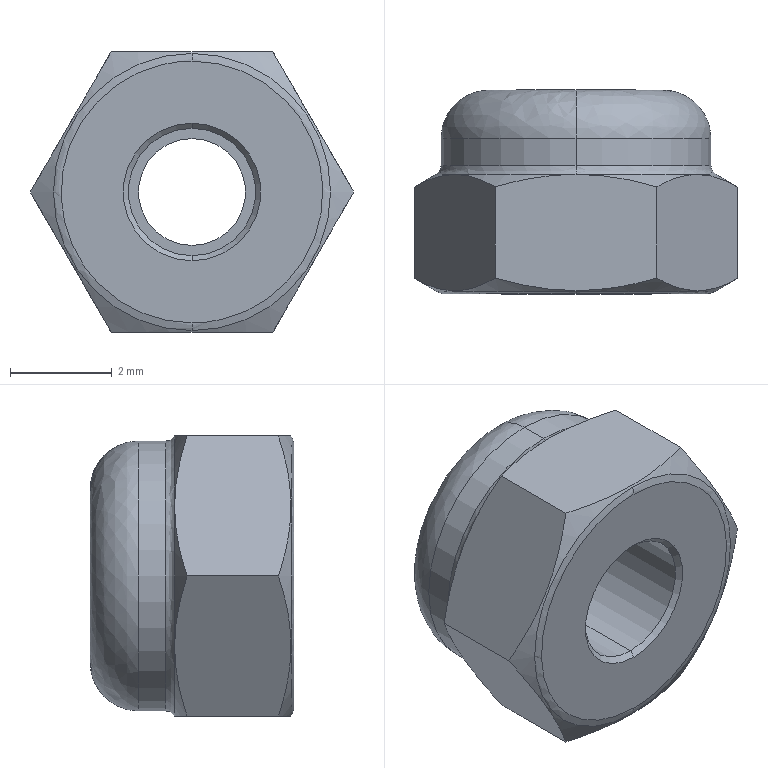Part | SolidWorks | features BaseBody 1 | 1 solid | 39 faces | box 6.351 x 4 x 5.5 mm | volume 76.032 mm3 | plane 11 | cone 10 | cylinder 10 | spline 8 | commonest cylinder face diameters 2.1 x2 2.5 x2 3 x2 4 x2 5.3 x2
STEP:
#1=CARTESIAN_POINT('',(0.,-1.16,2.72));
#2=VERTEX_POINT('',#1);
#3=CARTESIAN_POINT('',(0.,-1.16,-2.72));
#4=VERTEX_POINT('',#3);
#5=CARTESIAN_POINT('',(0.,-1.16,0.));
#6=DIRECTION('',(0.,-1.,0.));
#7=DIRECTION('',(0.,0.,1.));
#8=AXIS2_PLACEMENT_3D('',#5,#6,#7);
#9=CIRCLE('',#8,2.72);
#10=EDGE_CURVE('',#2,#4,#9,.T.);
#11=ORIENTED_EDGE('',*,*,#10,.T.);
#12=CARTESIAN_POINT('',(0.,-1.2,-2.57));
#13=VERTEX_POINT('',#12);
#14=CARTESIAN_POINT('',(0.,-0.9,-2.57));
#15=DIRECTION('',(-1.,0.,0.));
#16=DIRECTION('',(0.,0.,-1.));
#17=AXIS2_PLACEMENT_3D('',#14,#15,#16);
#18=CIRCLE('',#17,0.3);
#19=EDGE_CURVE('',#4,#13,#18,.T.);
#20=ORIENTED_EDGE('',*,*,#19,.T.);
#21=CARTESIAN_POINT('',(0.,-1.2,2.57));
#22=VERTEX_POINT('',#21);
#23=CARTESIAN_POINT('',(0.,-1.2,-2.57));
#24=CARTESIAN_POINT('',(-5.139,-1.2,-2.57));
#25=CARTESIAN_POINT('',(-5.139,-1.2,2.57));
#26=CARTESIAN_POINT('',(0.,-1.2,2.57));
#27=(BOUNDED_CURVE()B_SPLINE_CURVE(3,(#23,#24,#25,#26),.UNSPECIFIED.,.F.,.F.)B_SPLINE_CURVE_WITH_KNOTS((4,4),(0.,1.),.UNSPECIFIED.)CURVE()GEOMETRIC_REPRESENTATION_ITEM()RATIONAL_B_SPLINE_CURVE((1.,0.3333,0.3333,1.))REPRESENTATION_ITEM(''));
#28=EDGE_CURVE('',#13,#22,#27,.T.);
#29=ORIENTED_EDGE('',*,*,#28,.T.);
#30=CARTESIAN_POINT('',(0.,-0.9,2.57));
#31=DIRECTION('',(1.,0.,0.));
#32=DIRECTION('',(0.,0.,1.));
#33=AXIS2_PLACEMENT_3D('',#30,#31,#32);
#34=CIRCLE('',#33,0.3);
#35=EDGE_CURVE('',#2,#22,#34,.T.);
#36=ORIENTED_EDGE('',*,*,#35,.F.);
#37=EDGE_LOOP('',(#11,#20,#29,#36));
#38=FACE_OUTER_BOUND('',#37,.T.);
#39=CARTESIAN_POINT('',(0.,-1.16,-2.72));
#40=CARTESIAN_POINT('',(-5.439,-1.16,-2.72));
#41=CARTESIAN_POINT('',(-5.439,-1.16,2.72));
#42=CARTESIAN_POINT('',(0.,-1.16,2.72));
#43=CARTESIAN_POINT('',(0.,-1.186,-2.674));
#44=CARTESIAN_POINT('',(-5.347,-1.186,-2.674));
#45=CARTESIAN_POINT('',(-5.347,-1.186,2.674));
#46=CARTESIAN_POINT('',(0.,-1.186,2.674));
#47=CARTESIAN_POINT('',(0.,-1.2,-2.623));
#48=CARTESIAN_POINT('',(-5.245,-1.2,-2.623));
#49=CARTESIAN_POINT('',(-5.245,-1.2,2.623));
#50=CARTESIAN_POINT('',(0.,-1.2,2.623));
#51=CARTESIAN_POINT('',(0.,-1.2,-2.57));
#52=CARTESIAN_POINT('',(-5.139,-1.2,-2.57));
#53=CARTESIAN_POINT('',(-5.139,-1.2,2.57));
#54=CARTESIAN_POINT('',(0.,-1.2,2.57));
#55=(BOUNDED_SURFACE()B_SPLINE_SURFACE(3,3,((#39,#40,#41,#42),(#43,#44,#45,#46),(#47,#48,#49,#50),(#51,#52,#53,#54)),.UNSPECIFIED.,.F.,.F.,.F.)B_SPLINE_SURFACE_WITH_KNOTS((4,4),(4,4),(0.,1.),(0.,1.),.UNSPECIFIED.)GEOMETRIC_REPRESENTATION_ITEM()RATIONAL_B_SPLINE_SURFACE(((1.,0.3333,0.3333,1.),(0.9773,0.3258,0.3258,0.9773),(0.9773,0.3258,0.3258,0.9773),(1.,0.3333,0.3333,1.)))REPRESENTATION_ITEM('')SURFACE());
#56=ADVANCED_FACE('',(#38),#55,.T.);
#57=CARTESIAN_POINT('',(0.,1.142,-2.75));
#58=VERTEX_POINT('',#57);
#59=CARTESIAN_POINT('',(2.382,1.142,-1.375));
#60=VERTEX_POINT('',#59);
#61=CARTESIAN_POINT('',(0.,1.142,0.));
#62=DIRECTION('',(0.,-1.,0.));
#63=DIRECTION('',(0.,0.,-1.));
#64=AXIS2_PLACEMENT_3D('',#61,#62,#63);
#65=CIRCLE('',#64,2.75);
#66=EDGE_CURVE('',#58,#60,#65,.T.);
#67=ORIENTED_EDGE('',*,*,#66,.F.);
#68=CARTESIAN_POINT('',(0.,1.315,-2.65));
#69=VERTEX_POINT('',#68);
#70=CARTESIAN_POINT('',(0.,1.315,-2.85));
#71=DIRECTION('',(-1.,0.,0.));
#72=DIRECTION('',(0.,0.,-1.));
#73=AXIS2_PLACEMENT_3D('',#70,#71,#72);
#74=CIRCLE('',#73,0.2);
#75=EDGE_CURVE('',#58,#69,#74,.T.);
#76=ORIENTED_EDGE('',*,*,#75,.T.);
#77=CARTESIAN_POINT('',(0.,1.315,2.65));
#78=VERTEX_POINT('',#77);
#79=CARTESIAN_POINT('',(0.,1.315,0.));
#80=DIRECTION('',(0.,1.,0.));
#81=DIRECTION('',(0.,0.,1.));
#82=AXIS2_PLACEMENT_3D('',#79,#80,#81);
#83=CIRCLE('',#82,2.65);
#84=EDGE_CURVE('',#78,#69,#83,.T.);
#85=ORIENTED_EDGE('',*,*,#84,.F.);
#86=CARTESIAN_POINT('',(0.,1.142,2.75));
#87=VERTEX_POINT('',#86);
#88=CARTESIAN_POINT('',(0.,1.315,2.85));
#89=DIRECTION('',(1.,0.,0.));
#90=DIRECTION('',(0.,0.,1.));
#91=AXIS2_PLACEMENT_3D('',#88,#89,#90);
#92=CIRCLE('',#91,0.2);
#93=EDGE_CURVE('',#87,#78,#92,.T.);
#94=ORIENTED_EDGE('',*,*,#93,.F.);
#95=CARTESIAN_POINT('',(2.382,1.142,1.375));
#96=VERTEX_POINT('',#95);
#97=CARTESIAN_POINT('',(0.,1.142,0.));
#98=DIRECTION('',(0.,-1.,0.));
#99=DIRECTION('',(0.,0.,1.));
#100=AXIS2_PLACEMENT_3D('',#97,#98,#99);
#101=CIRCLE('',#100,2.75);
#102=EDGE_CURVE('',#96,#87,#101,.T.);
#103=ORIENTED_EDGE('',*,*,#102,.F.);
#104=CARTESIAN_POINT('',(0.,1.142,0.));
#105=DIRECTION('',(0.,-1.,0.));
#106=DIRECTION('',(0.,0.,1.));
#107=AXIS2_PLACEMENT_3D('',#104,#105,#106);
#108=CIRCLE('',#107,2.75);
#109=EDGE_CURVE('',#60,#96,#108,.T.);
#110=ORIENTED_EDGE('',*,*,#109,.F.);
#111=EDGE_LOOP('',(#67,#76,#85,#94,#103,#110));
#112=FACE_OUTER_BOUND('',#111,.T.);
#113=CARTESIAN_POINT('',(0.,1.142,2.75));
#114=CARTESIAN_POINT('',(5.5,1.142,2.75));
#115=CARTESIAN_POINT('',(5.5,1.142,-2.75));
#116=CARTESIAN_POINT('',(0.,1.142,-2.75));
#117=CARTESIAN_POINT('',(0.,1.179,2.687));
#118=CARTESIAN_POINT('',(5.373,1.179,2.687));
#119=CARTESIAN_POINT('',(5.373,1.179,-2.687));
#120=CARTESIAN_POINT('',(0.,1.179,-2.687));
#121=CARTESIAN_POINT('',(0.,1.242,2.65));
#122=CARTESIAN_POINT('',(5.3,1.242,2.65));
#123=CARTESIAN_POINT('',(5.3,1.242,-2.65));
#124=CARTESIAN_POINT('',(0.,1.242,-2.65));
#125=CARTESIAN_POINT('',(0.,1.315,2.65));
#126=CARTESIAN_POINT('',(5.3,1.315,2.65));
#127=CARTESIAN_POINT('',(5.3,1.315,-2.65));
#128=CARTESIAN_POINT('',(0.,1.315,-2.65));
#129=(BOUNDED_SURFACE()B_SPLINE_SURFACE(3,3,((#113,#114,#115,#116),(#117,#118,#119,#120),(#121,#122,#123,#124),(#125,#126,#127,#128)),.UNSPECIFIED.,.F.,.F.,.F.)B_SPLINE_SURFACE_WITH_KNOTS((4,4),(4,4),(0.,1.),(0.,1.),.UNSPECIFIED.)GEOMETRIC_REPRESENTATION_ITEM()RATIONAL_B_SPLINE_SURFACE(((1.,0.3333,0.3333,1.),(0.9107,0.3036,0.3036,0.9107),(0.9107,0.3036,0.3036,0.9107),(1.,0.3333,0.3333,1.)))REPRESENTATION_ITEM('')SURFACE());
#130=ADVANCED_FACE('',(#112),#129,.F.);
#131=CARTESIAN_POINT('',(0.,2.8,-1.7));
#132=VERTEX_POINT('',#131);
#133=CARTESIAN_POINT('',(0.,2.8,1.7));
#134=VERTEX_POINT('',#133);
#135=CARTESIAN_POINT('',(0.,2.8,-1.7));
#136=CARTESIAN_POINT('',(-0.108,2.8,-1.7));
#137=CARTESIAN_POINT('',(-0.2672,2.8,-1.685));
#138=CARTESIAN_POINT('',(-0.4481,2.8,-1.642));
#139=CARTESIAN_POINT('',(-0.5373,2.8,-1.613));
#140=CARTESIAN_POINT('',(-0.5753,2.8,-1.6));
#141=CARTESIAN_POINT('',(-0.6006,2.8,-1.59));
#142=CARTESIAN_POINT('',(-0.6121,2.8,-1.586));
#143=CARTESIAN_POINT('',(-0.8437,2.8,-1.494));
#144=CARTESIAN_POINT('',(-1.036,2.8,-1.368));
#145=CARTESIAN_POINT('',(-1.285,2.8,-1.119));
#146=CARTESIAN_POINT('',(-1.394,2.8,-0.9851));
#147=CARTESIAN_POINT('',(-1.496,2.8,-0.8112));
#148=CARTESIAN_POINT('',(-1.541,2.8,-0.7199));
#149=CARTESIAN_POINT('',(-1.558,2.8,-0.6799));
#150=CARTESIAN_POINT('',(-1.57,2.8,-0.653));
#151=CARTESIAN_POINT('',(-1.576,2.8,-0.6383));
#152=CARTESIAN_POINT('',(-1.66,2.8,-0.4251));
#153=CARTESIAN_POINT('',(-1.7,2.8,-0.2158));
#154=CARTESIAN_POINT('',(-1.7,2.8,0.1079));
#155=CARTESIAN_POINT('',(-1.685,2.8,0.2671));
#156=CARTESIAN_POINT('',(-1.642,2.8,0.448));
#157=CARTESIAN_POINT('',(-1.617,2.8,0.5245));
#158=CARTESIAN_POINT('',(-1.6,2.8,0.5753));
#159=CARTESIAN_POINT('',(-1.591,2.8,0.5985));
#160=CARTESIAN_POINT('',(-1.494,2.8,0.8437));
#161=CARTESIAN_POINT('',(-1.368,2.8,1.036));
#162=CARTESIAN_POINT('',(-1.119,2.8,1.285));
#163=CARTESIAN_POINT('',(-0.9851,2.8,1.394));
#164=CARTESIAN_POINT('',(-0.8112,2.8,1.496));
#165=CARTESIAN_POINT('',(-0.7199,2.8,1.541));
#166=CARTESIAN_POINT('',(-0.6799,2.8,1.558));
#167=CARTESIAN_POINT('',(-0.653,2.8,1.57));
#168=CARTESIAN_POINT('',(-0.6383,2.8,1.576));
#169=CARTESIAN_POINT('',(-0.4249,2.8,1.66));
#170=CARTESIAN_POINT('',(-0.2164,2.8,1.7));
#171=CARTESIAN_POINT('',(0.,2.8,1.7));
#172=B_SPLINE_CURVE_WITH_KNOTS('',3,(#135,#136,#137,#138,#139,#140,#141,#142,#143,#144,#145,#146,#147,#148,#149,#150,#151,#152,#153,#154,#155,#156,#157,#158,#159,#160,#161,#162,#163,#164,#165,#166,#167,#168,#169,#170,#171),.UNSPECIFIED.,.F.,.F.,(4,1,1,1,2,2,2,1,1,1,2,2,2,1,1,2,2,2,1,1,1,2,2,4),(0.,0.0625,0.09375,0.1094,0.1172,0.125,0.25,0.3125,0.3438,0.3594,0.3672,0.375,0.5,0.5625,0.5938,0.6094,0.625,0.75,0.8125,0.8438,0.8594,0.8672,0.875,1.),.UNSPECIFIED.);
#173=EDGE_CURVE('',#132,#134,#172,.T.);
#174=ORIENTED_EDGE('',*,*,#173,.F.);
#175=CARTESIAN_POINT('',(0.,1.85,-2.65));
#176=VERTEX_POINT('',#175);
#177=CARTESIAN_POINT('',(0.,1.85,-1.7));
#178=DIRECTION('',(-1.,0.,0.));
#179=DIRECTION('',(0.,0.,-1.));
#180=AXIS2_PLACEMENT_3D('',#177,#178,#179);
#181=CIRCLE('',#180,0.95);
#182=EDGE_CURVE('',#132,#176,#181,.T.);
#183=ORIENTED_EDGE('',*,*,#182,.T.);
#184=CARTESIAN_POINT('',(0.,1.85,2.65));
#185=VERTEX_POINT('',#184);
#186=CARTESIAN_POINT('',(0.,1.85,0.));
#187=DIRECTION('',(0.,-1.,0.));
#188=DIRECTION('',(0.,0.,1.));
#189=AXIS2_PLACEMENT_3D('',#186,#187,#188);
#190=CIRCLE('',#189,2.65);
#191=EDGE_CURVE('',#185,#176,#190,.T.);
#192=ORIENTED_EDGE('',*,*,#191,.F.);
#193=CARTESIAN_POINT('',(0.,1.85,1.7));
#194=DIRECTION('',(1.,0.,0.));
#195=DIRECTION('',(0.,0.,1.));
#196=AXIS2_PLACEMENT_3D('',#193,#194,#195);
#197=CIRCLE('',#196,0.95);
#198=EDGE_CURVE('',#134,#185,#197,.T.);
#199=ORIENTED_EDGE('',*,*,#198,.F.);
#200=EDGE_LOOP('',(#174,#183,#192,#199));
#201=FACE_OUTER_BOUND('',#200,.T.);
#202=CARTESIAN_POINT('',(0.,2.8,-1.7));
#203=CARTESIAN_POINT('',(-3.4,2.8,-1.7));
#204=CARTESIAN_POINT('',(-3.4,2.8,1.7));
#205=CARTESIAN_POINT('',(0.,2.8,1.7));
#206=CARTESIAN_POINT('',(0.,2.8,-2.256));
#207=CARTESIAN_POINT('',(-4.513,2.8,-2.256));
#208=CARTESIAN_POINT('',(-4.513,2.8,2.256));
#209=CARTESIAN_POINT('',(0.,2.8,2.256));
#210=CARTESIAN_POINT('',(0.,2.406,-2.65));
#211=CARTESIAN_POINT('',(-5.3,2.406,-2.65));
#212=CARTESIAN_POINT('',(-5.3,2.406,2.65));
#213=CARTESIAN_POINT('',(0.,2.406,2.65));
#214=CARTESIAN_POINT('',(0.,1.85,-2.65));
#215=CARTESIAN_POINT('',(-5.3,1.85,-2.65));
#216=CARTESIAN_POINT('',(-5.3,1.85,2.65));
#217=CARTESIAN_POINT('',(0.,1.85,2.65));
#218=(BOUNDED_SURFACE()B_SPLINE_SURFACE(3,3,((#202,#203,#204,#205),(#206,#207,#208,#209),(#210,#211,#212,#213),(#214,#215,#216,#217)),.UNSPECIFIED.,.F.,.F.,.F.)B_SPLINE_SURFACE_WITH_KNOTS((4,4),(4,4),(0.,1.),(0.,1.),.UNSPECIFIED.)GEOMETRIC_REPRESENTATION_ITEM()RATIONAL_B_SPLINE_SURFACE(((1.,0.3333,0.3333,1.),(0.8047,0.2682,0.2682,0.8047),(0.8047,0.2682,0.2682,0.8047),(1.,0.3333,0.3333,1.)))REPRESENTATION_ITEM('')SURFACE());
#219=ADVANCED_FACE('',(#201),#218,.T.);
#220=CARTESIAN_POINT('',(0.,2.65,1.5));
#221=VERTEX_POINT('',#220);
#222=CARTESIAN_POINT('',(0.,2.65,-1.5));
#223=VERTEX_POINT('',#222);
#224=CARTESIAN_POINT('',(0.,2.65,0.));
#225=DIRECTION('',(0.,-1.,0.));
#226=DIRECTION('',(0.,0.,1.));
#227=AXIS2_PLACEMENT_3D('',#224,#225,#226);
#228=CIRCLE('',#227,1.5);
#229=EDGE_CURVE('',#221,#223,#228,.T.);
#230=ORIENTED_EDGE('',*,*,#229,.T.);
#231=CARTESIAN_POINT('',(0.,2.8,-1.65));
#232=VERTEX_POINT('',#231);
#233=CARTESIAN_POINT('',(0.,2.65,-1.65));
#234=DIRECTION('',(-1.,0.,0.));
#235=DIRECTION('',(0.,0.,-1.));
#236=AXIS2_PLACEMENT_3D('',#233,#234,#235);
#237=CIRCLE('',#236,0.15);
#238=EDGE_CURVE('',#223,#232,#237,.T.);
#239=ORIENTED_EDGE('',*,*,#238,.T.);
#240=CARTESIAN_POINT('',(0.,2.8,1.65));
#241=VERTEX_POINT('',#240);
#242=CARTESIAN_POINT('',(0.,2.8,1.65));
#243=CARTESIAN_POINT('',(-0.1048,2.8,1.65));
#244=CARTESIAN_POINT('',(-0.2594,2.8,1.636));
#245=CARTESIAN_POINT('',(-0.4349,2.8,1.593));
#246=CARTESIAN_POINT('',(-0.5092,2.8,1.57));
#247=CARTESIAN_POINT('',(-0.5584,2.8,1.553));
#248=CARTESIAN_POINT('',(-0.5809,2.8,1.545));
#249=CARTESIAN_POINT('',(-0.8189,2.8,1.45));
#250=CARTESIAN_POINT('',(-1.006,2.8,1.328));
#251=CARTESIAN_POINT('',(-1.247,2.8,1.086));
#252=CARTESIAN_POINT('',(-1.353,2.8,0.9561));
#253=CARTESIAN_POINT('',(-1.452,2.8,0.7873));
#254=CARTESIAN_POINT('',(-1.495,2.8,0.6988));
#255=CARTESIAN_POINT('',(-1.512,2.8,0.6599));
#256=CARTESIAN_POINT('',(-1.523,2.8,0.6338));
#257=CARTESIAN_POINT('',(-1.529,2.8,0.6195));
#258=CARTESIAN_POINT('',(-1.611,2.8,0.4126));
#259=CARTESIAN_POINT('',(-1.65,2.8,0.2095));
#260=CARTESIAN_POINT('',(-1.65,2.8,-0.1047));
#261=CARTESIAN_POINT('',(-1.636,2.8,-0.2592));
#262=CARTESIAN_POINT('',(-1.593,2.8,-0.4348));
#263=CARTESIAN_POINT('',(-1.57,2.8,-0.5091));
#264=CARTESIAN_POINT('',(-1.553,2.8,-0.5584));
#265=CARTESIAN_POINT('',(-1.545,2.8,-0.5809));
#266=CARTESIAN_POINT('',(-1.45,2.8,-0.8189));
#267=CARTESIAN_POINT('',(-1.328,2.8,-1.006));
#268=CARTESIAN_POINT('',(-1.086,2.8,-1.247));
#269=CARTESIAN_POINT('',(-0.9561,2.8,-1.353));
#270=CARTESIAN_POINT('',(-0.7873,2.8,-1.452));
#271=CARTESIAN_POINT('',(-0.6988,2.8,-1.495));
#272=CARTESIAN_POINT('',(-0.6599,2.8,-1.512));
#273=CARTESIAN_POINT('',(-0.6338,2.8,-1.523));
#274=CARTESIAN_POINT('',(-0.6195,2.8,-1.529));
#275=CARTESIAN_POINT('',(-0.4124,2.8,-1.611));
#276=CARTESIAN_POINT('',(-0.21,2.8,-1.65));
#277=CARTESIAN_POINT('',(0.,2.8,-1.65));
#278=B_SPLINE_CURVE_WITH_KNOTS('',3,(#242,#243,#244,#245,#246,#247,#248,#249,#250,#251,#252,#253,#254,#255,#256,#257,#258,#259,#260,#261,#262,#263,#264,#265,#266,#267,#268,#269,#270,#271,#272,#273,#274,#275,#276,#277),.UNSPECIFIED.,.F.,.F.,(4,1,1,2,2,2,1,1,1,2,2,2,1,1,2,2,2,1,1,1,2,2,4),(0.,0.0625,0.09375,0.1094,0.125,0.25,0.3125,0.3438,0.3594,0.3672,0.375,0.5,0.5625,0.5938,0.6094,0.625,0.75,0.8125,0.8438,0.8594,0.8672,0.875,1.),.UNSPECIFIED.);
#279=EDGE_CURVE('',#241,#232,#278,.T.);
#280=ORIENTED_EDGE('',*,*,#279,.F.);
#281=CARTESIAN_POINT('',(0.,2.65,1.65));
#282=DIRECTION('',(1.,0.,0.));
#283=DIRECTION('',(0.,0.,1.));
#284=AXIS2_PLACEMENT_3D('',#281,#282,#283);
#285=CIRCLE('',#284,0.15);
#286=EDGE_CURVE('',#221,#241,#285,.T.);
#287=ORIENTED_EDGE('',*,*,#286,.F.);
#288=EDGE_LOOP('',(#230,#239,#280,#287));
#289=FACE_OUTER_BOUND('',#288,.T.);
#290=CARTESIAN_POINT('',(0.,2.65,-1.5));
#291=CARTESIAN_POINT('',(-3.,2.65,-1.5));
#292=CARTESIAN_POINT('',(-3.,2.65,1.5));
#293=CARTESIAN_POINT('',(0.,2.65,1.5));
#294=CARTESIAN_POINT('',(0.,2.738,-1.5));
#295=CARTESIAN_POINT('',(-3.,2.738,-1.5));
#296=CARTESIAN_POINT('',(-3.,2.738,1.5));
#297=CARTESIAN_POINT('',(0.,2.738,1.5));
#298=CARTESIAN_POINT('',(0.,2.8,-1.562));
#299=CARTESIAN_POINT('',(-3.124,2.8,-1.562));
#300=CARTESIAN_POINT('',(-3.124,2.8,1.562));
#301=CARTESIAN_POINT('',(0.,2.8,1.562));
#302=CARTESIAN_POINT('',(0.,2.8,-1.65));
#303=CARTESIAN_POINT('',(-3.3,2.8,-1.65));
#304=CARTESIAN_POINT('',(-3.3,2.8,1.65));
#305=CARTESIAN_POINT('',(0.,2.8,1.65));
#306=(BOUNDED_SURFACE()B_SPLINE_SURFACE(3,3,((#290,#291,#292,#293),(#294,#295,#296,#297),(#298,#299,#300,#301),(#302,#303,#304,#305)),.UNSPECIFIED.,.F.,.F.,.F.)B_SPLINE_SURFACE_WITH_KNOTS((4,4),(4,4),(0.,1.),(0.,1.),.UNSPECIFIED.)GEOMETRIC_REPRESENTATION_ITEM()RATIONAL_B_SPLINE_SURFACE(((1.,0.3333,0.3333,1.),(0.8047,0.2682,0.2682,0.8047),(0.8047,0.2682,0.2682,0.8047),(1.,0.3333,0.3333,1.)))REPRESENTATION_ITEM('')SURFACE());
#307=ADVANCED_FACE('',(#289),#306,.T.);
#308=CARTESIAN_POINT('',(0.,-1.1,1.25));
#309=VERTEX_POINT('',#308);
#310=CARTESIAN_POINT('',(0.,-1.1,-1.25));
#311=VERTEX_POINT('',#310);
#312=CARTESIAN_POINT('',(0.,-1.1,0.));
#313=DIRECTION('',(0.,-1.,0.));
#314=DIRECTION('',(0.,0.,-1.));
#315=AXIS2_PLACEMENT_3D('',#312,#313,#314);
#316=CIRCLE('',#315,1.25);
#317=EDGE_CURVE('',#309,#311,#316,.T.);
#318=ORIENTED_EDGE('',*,*,#317,.F.);
#319=CARTESIAN_POINT('',(0.,-1.2,1.35));
#320=VERTEX_POINT('',#319);
#321=CARTESIAN_POINT('',(0.,-1.2,1.35));
#322=DIRECTION('',(0.,-0.7071,0.7071));
#323=VECTOR('',#322,1000.);
#324=LINE('',#321,#323);
#325=EDGE_CURVE('',#309,#320,#324,.T.);
#326=ORIENTED_EDGE('',*,*,#325,.T.);
#327=CARTESIAN_POINT('',(0.,-1.2,-1.35));
#328=VERTEX_POINT('',#327);
#329=CARTESIAN_POINT('',(0.,-1.2,0.));
#330=DIRECTION('',(0.,-1.,0.));
#331=DIRECTION('',(0.,0.,-1.));
#332=AXIS2_PLACEMENT_3D('',#329,#330,#331);
#333=CIRCLE('',#332,1.35);
#334=EDGE_CURVE('',#320,#328,#333,.T.);
#335=ORIENTED_EDGE('',*,*,#334,.T.);
#336=CARTESIAN_POINT('',(0.,-1.2,-1.35));
#337=DIRECTION('',(0.,-0.7071,-0.7071));
#338=VECTOR('',#337,1000.);
#339=LINE('',#336,#338);
#340=EDGE_CURVE('',#311,#328,#339,.T.);
#341=ORIENTED_EDGE('',*,*,#340,.F.);
#342=EDGE_LOOP('',(#318,#326,#335,#341));
#343=FACE_OUTER_BOUND('',#342,.T.);
#344=CARTESIAN_POINT('',(0.,-1.2,0.));
#345=DIRECTION('',(0.,-1.,0.));
#346=DIRECTION('',(0.,0.,-1.));
#347=AXIS2_PLACEMENT_3D('',#344,#345,#346);
#348=CONICAL_SURFACE('',#347,1.35,0.7854);
#349=ADVANCED_FACE('',(#343),#348,.F.);
#350=CARTESIAN_POINT('',(0.,-1.16,0.));
#351=DIRECTION('',(0.,-1.,0.));
#352=DIRECTION('',(0.,0.,1.));
#353=AXIS2_PLACEMENT_3D('',#350,#351,#352);
#354=CIRCLE('',#353,2.72);
#355=EDGE_CURVE('',#4,#2,#354,.T.);
#356=ORIENTED_EDGE('',*,*,#355,.F.);
#357=CARTESIAN_POINT('',(0.,-1.142,-2.75));
#358=VERTEX_POINT('',#357);
#359=CARTESIAN_POINT('',(0.,-0.8951,-3.178));
#360=DIRECTION('',(0.,0.5,-0.866));
#361=VECTOR('',#360,1000.);
#362=LINE('',#359,#361);
#363=EDGE_CURVE('',#4,#358,#362,.T.);
#364=ORIENTED_EDGE('',*,*,#363,.T.);
#365=CARTESIAN_POINT('',(1.588,-0.8966,-2.75));
#366=VERTEX_POINT('',#365);
#367=CARTESIAN_POINT('',(0.,-1.142,-2.75));
#368=CARTESIAN_POINT('',(0.5419,-1.142,-2.75));
#369=CARTESIAN_POINT('',(1.069,-1.046,-2.75));
#370=CARTESIAN_POINT('',(1.588,-0.8966,-2.75));
#371=B_SPLINE_CURVE_WITH_KNOTS('',3,(#367,#368,#369,#370),.UNSPECIFIED.,.F.,.F.,(4,4),(0.001607,0.003213),.UNSPECIFIED.);
#372=EDGE_CURVE('',#358,#366,#371,.T.);
#373=ORIENTED_EDGE('',*,*,#372,.T.);
#374=CARTESIAN_POINT('',(3.175,-0.8966,-0.000000043));
#375=VERTEX_POINT('',#374);
#376=CARTESIAN_POINT('',(1.588,-0.8966,-2.75));
#377=CARTESIAN_POINT('',(1.847,-1.046,-2.301));
#378=CARTESIAN_POINT('',(2.11,-1.142,-1.845));
#379=CARTESIAN_POINT('',(2.515,-1.142,-1.144));
#380=CARTESIAN_POINT('',(2.65,-1.119,-0.9103));
#381=CARTESIAN_POINT('',(2.915,-1.033,-0.4515));
#382=CARTESIAN_POINT('',(3.046,-0.9716,-0.2248));
#383=CARTESIAN_POINT('',(3.175,-0.8966,-0.000000043));
#384=B_SPLINE_CURVE_WITH_KNOTS('',3,(#376,#377,#378,#379,#380,#381,#382,#383),.UNSPECIFIED.,.F.,.F.,(4,2,2,4),(0.,0.001604,0.002405,0.003207),.UNSPECIFIED.);
#385=EDGE_CURVE('',#366,#375,#384,.T.);
#386=ORIENTED_EDGE('',*,*,#385,.T.);
#387=CARTESIAN_POINT('',(1.588,-0.8966,2.75));
#388=VERTEX_POINT('',#387);
#389=CARTESIAN_POINT('',(3.175,-0.8966,-0.000000043));
#390=CARTESIAN_POINT('',(2.916,-1.046,0.449));
#391=CARTESIAN_POINT('',(2.653,-1.142,0.9048));
#392=CARTESIAN_POINT('',(2.248,-1.142,1.606));
#393=CARTESIAN_POINT('',(2.113,-1.119,1.84));
#394=CARTESIAN_POINT('',(1.848,-1.033,2.299));
#395=CARTESIAN_POINT('',(1.717,-0.9716,2.525));
#396=CARTESIAN_POINT('',(1.588,-0.8966,2.75));
#397=B_SPLINE_CURVE_WITH_KNOTS('',3,(#389,#390,#391,#392,#393,#394,#395,#396),.UNSPECIFIED.,.F.,.F.,(4,2,2,4),(0.,0.001604,0.002405,0.003207),.UNSPECIFIED.);
#398=EDGE_CURVE('',#375,#388,#397,.T.);
#399=ORIENTED_EDGE('',*,*,#398,.T.);
#400=CARTESIAN_POINT('',(0.,-1.142,2.75));
#401=VERTEX_POINT('',#400);
#402=CARTESIAN_POINT('',(1.588,-0.8966,2.75));
#403=CARTESIAN_POINT('',(1.069,-1.046,2.75));
#404=CARTESIAN_POINT('',(0.5419,-1.142,2.75));
#405=CARTESIAN_POINT('',(0.,-1.142,2.75));
#406=B_SPLINE_CURVE_WITH_KNOTS('',3,(#402,#403,#404,#405),.UNSPECIFIED.,.F.,.F.,(4,4),(0.,0.001607),.UNSPECIFIED.);
#407=EDGE_CURVE('',#388,#401,#406,.T.);
#408=ORIENTED_EDGE('',*,*,#407,.T.);
#409=CARTESIAN_POINT('',(0.,-0.8951,3.178));
#410=DIRECTION('',(0.,0.5,0.866));
#411=VECTOR('',#410,1000.);
#412=LINE('',#409,#411);
#413=EDGE_CURVE('',#2,#401,#412,.T.);
#414=ORIENTED_EDGE('',*,*,#413,.F.);
#415=EDGE_LOOP('',(#356,#364,#373,#386,#399,#408,#414));
#416=FACE_OUTER_BOUND('',#415,.T.);
#417=CARTESIAN_POINT('',(0.,-0.8951,0.));
#418=DIRECTION('',(0.,1.,0.));
#419=DIRECTION('',(0.,0.,1.));
#420=AXIS2_PLACEMENT_3D('',#417,#418,#419);
#421=CONICAL_SURFACE('',#420,3.178,1.047);
#422=ADVANCED_FACE('',(#416),#421,.T.);
#423=CARTESIAN_POINT('',(0.,1.2,1.25));
#424=VERTEX_POINT('',#423);
#425=CARTESIAN_POINT('',(0.,1.2,-1.25));
#426=VERTEX_POINT('',#425);
#427=CARTESIAN_POINT('',(0.,1.2,0.));
#428=DIRECTION('',(0.,-1.,0.));
#429=DIRECTION('',(0.,0.,-1.));
#430=AXIS2_PLACEMENT_3D('',#427,#428,#429);
#431=CIRCLE('',#430,1.25);
#432=EDGE_CURVE('',#424,#426,#431,.T.);
#433=ORIENTED_EDGE('',*,*,#432,.F.);
#434=CARTESIAN_POINT('',(0.,1.2,1.25));
#435=DIRECTION('',(0.,-1.,0.));
#436=VECTOR('',#435,1000.);
#437=LINE('',#434,#436);
#438=EDGE_CURVE('',#424,#309,#437,.T.);
#439=ORIENTED_EDGE('',*,*,#438,.T.);
#440=ORIENTED_EDGE('',*,*,#317,.T.);
#441=CARTESIAN_POINT('',(0.,1.2,-1.25));
#442=DIRECTION('',(0.,-1.,0.));
#443=VECTOR('',#442,1000.);
#444=LINE('',#441,#443);
#445=EDGE_CURVE('',#426,#311,#444,.T.);
#446=ORIENTED_EDGE('',*,*,#445,.F.);
#447=EDGE_LOOP('',(#433,#439,#440,#446));
#448=FACE_OUTER_BOUND('',#447,.T.);
#449=CARTESIAN_POINT('',(0.,1.2,0.));
#450=DIRECTION('',(0.,-1.,0.));
#451=DIRECTION('',(0.,0.,-1.));
#452=AXIS2_PLACEMENT_3D('',#449,#450,#451);
#453=CYLINDRICAL_SURFACE('',#452,1.25);
#454=ADVANCED_FACE('',(#448),#453,.F.);
#455=CARTESIAN_POINT('',(0.,1.2,-1.05));
#456=VERTEX_POINT('',#455);
#457=CARTESIAN_POINT('',(0.,1.2,1.05));
#458=VERTEX_POINT('',#457);
#459=CARTESIAN_POINT('',(0.,1.2,0.));
#460=DIRECTION('',(0.,1.,0.));
#461=DIRECTION('',(0.,0.,1.));
#462=AXIS2_PLACEMENT_3D('',#459,#460,#461);
#463=CIRCLE('',#462,1.05);
#464=EDGE_CURVE('',#456,#458,#463,.T.);
#465=ORIENTED_EDGE('',*,*,#464,.F.);
#466=CARTESIAN_POINT('',(0.,2.523,-1.05));
#467=VERTEX_POINT('',#466);
#468=CARTESIAN_POINT('',(0.,2.514,-1.05));
#469=DIRECTION('',(0.,1.,0.));
#470=VECTOR('',#469,1000.);
#471=LINE('',#468,#470);
#472=EDGE_CURVE('',#456,#467,#471,.T.);
#473=ORIENTED_EDGE('',*,*,#472,.T.);
#474=CARTESIAN_POINT('',(0.,2.523,1.05));
#475=VERTEX_POINT('',#474);
#476=CARTESIAN_POINT('',(0.,2.523,0.));
#477=DIRECTION('',(0.,-1.,0.));
#478=DIRECTION('',(0.,0.,1.));
#479=AXIS2_PLACEMENT_3D('',#476,#477,#478);
#480=CIRCLE('',#479,1.05);
#481=EDGE_CURVE('',#475,#467,#480,.T.);
#482=ORIENTED_EDGE('',*,*,#481,.F.);
#483=CARTESIAN_POINT('',(0.,2.514,1.05));
#484=DIRECTION('',(0.,1.,0.));
#485=VECTOR('',#484,1000.);
#486=LINE('',#483,#485);
#487=EDGE_CURVE('',#458,#475,#486,.T.);
#488=ORIENTED_EDGE('',*,*,#487,.F.);
#489=EDGE_LOOP('',(#465,#473,#482,#488));
#490=FACE_OUTER_BOUND('',#489,.T.);
#491=CARTESIAN_POINT('',(0.,2.514,0.));
#492=DIRECTION('',(0.,1.,0.));
#493=DIRECTION('',(0.,0.,1.));
#494=AXIS2_PLACEMENT_3D('',#491,#492,#493);
#495=CYLINDRICAL_SURFACE('',#494,1.05);
#496=ADVANCED_FACE('',(#490),#495,.F.);
#497=ORIENTED_EDGE('',*,*,#84,.T.);
#498=CARTESIAN_POINT('',(0.,2.805,-2.65));
#499=DIRECTION('',(0.,1.,0.));
#500=VECTOR('',#499,1000.);
#501=LINE('',#498,#500);
#502=EDGE_CURVE('',#69,#176,#501,.T.);
#503=ORIENTED_EDGE('',*,*,#502,.T.);
#504=CARTESIAN_POINT('',(0.,1.85,0.));
#505=DIRECTION('',(0.,-1.,0.));
#506=DIRECTION('',(0.,0.,1.));
#507=AXIS2_PLACEMENT_3D('',#504,#505,#506);
#508=CIRCLE('',#507,2.65);
#509=EDGE_CURVE('',#176,#185,#508,.T.);
#510=ORIENTED_EDGE('',*,*,#509,.T.);
#511=CARTESIAN_POINT('',(0.,2.805,2.65));
#512=DIRECTION('',(0.,1.,0.));
#513=VECTOR('',#512,1000.);
#514=LINE('',#511,#513);
#515=EDGE_CURVE('',#78,#185,#514,.T.);
#516=ORIENTED_EDGE('',*,*,#515,.F.);
#517=EDGE_LOOP('',(#497,#503,#510,#516));
#518=FACE_OUTER_BOUND('',#517,.T.);
#519=CARTESIAN_POINT('',(0.,2.805,0.));
#520=DIRECTION('',(0.,1.,0.));
#521=DIRECTION('',(0.,0.,1.));
#522=AXIS2_PLACEMENT_3D('',#519,#520,#521);
#523=CYLINDRICAL_SURFACE('',#522,2.65);
#524=ADVANCED_FACE('',(#518),#523,.T.);
#525=CARTESIAN_POINT('',(0.,2.523,-2.));
#526=VERTEX_POINT('',#525);
#527=CARTESIAN_POINT('',(0.,2.523,2.));
#528=VERTEX_POINT('',#527);
#529=CARTESIAN_POINT('',(0.,2.523,0.));
#530=DIRECTION('',(0.,1.,0.));
#531=DIRECTION('',(0.,0.,1.));
#532=AXIS2_PLACEMENT_3D('',#529,#530,#531);
#533=CIRCLE('',#532,2.);
#534=EDGE_CURVE('',#526,#528,#533,.T.);
#535=ORIENTED_EDGE('',*,*,#534,.F.);
#536=CARTESIAN_POINT('',(0.,2.533,-2.));
#537=VERTEX_POINT('',#536);
#538=CARTESIAN_POINT('',(0.,2.805,-2.));
#539=DIRECTION('',(0.,1.,0.));
#540=VECTOR('',#539,1000.);
#541=LINE('',#538,#540);
#542=EDGE_CURVE('',#526,#537,#541,.T.);
#543=ORIENTED_EDGE('',*,*,#542,.T.);
#544=CARTESIAN_POINT('',(0.,2.533,2.));
#545=VERTEX_POINT('',#544);
#546=CARTESIAN_POINT('',(0.,2.533,0.));
#547=DIRECTION('',(0.,-1.,0.));
#548=DIRECTION('',(0.,0.,1.));
#549=AXIS2_PLACEMENT_3D('',#546,#547,#548);
#550=CIRCLE('',#549,2.);
#551=EDGE_CURVE('',#545,#537,#550,.T.);
#552=ORIENTED_EDGE('',*,*,#551,.F.);
#553=CARTESIAN_POINT('',(0.,2.805,2.));
#554=DIRECTION('',(0.,1.,0.));
#555=VECTOR('',#554,1000.);
#556=LINE('',#553,#555);
#557=EDGE_CURVE('',#528,#545,#556,.T.);
#558=ORIENTED_EDGE('',*,*,#557,.F.);
#559=EDGE_LOOP('',(#535,#543,#552,#558));
#560=FACE_OUTER_BOUND('',#559,.T.);
#561=CARTESIAN_POINT('',(0.,2.805,0.));
#562=DIRECTION('',(0.,1.,0.));
#563=DIRECTION('',(0.,0.,1.));
#564=AXIS2_PLACEMENT_3D('',#561,#562,#563);
#565=CYLINDRICAL_SURFACE('',#564,2.);
#566=ADVANCED_FACE('',(#560),#565,.F.);
#567=CARTESIAN_POINT('',(0.,2.533,-1.5));
#568=VERTEX_POINT('',#567);
#569=CARTESIAN_POINT('',(0.,2.533,1.5));
#570=VERTEX_POINT('',#569);
#571=CARTESIAN_POINT('',(0.,2.533,0.));
#572=DIRECTION('',(0.,1.,0.));
#573=DIRECTION('',(0.,0.,1.));
#574=AXIS2_PLACEMENT_3D('',#571,#572,#573);
#575=CIRCLE('',#574,1.5);
#576=EDGE_CURVE('',#568,#570,#575,.T.);
#577=ORIENTED_EDGE('',*,*,#576,.F.);
#578=CARTESIAN_POINT('',(0.,2.805,-1.5));
#579=DIRECTION('',(0.,1.,0.));
#580=VECTOR('',#579,1000.);
#581=LINE('',#578,#580);
#582=EDGE_CURVE('',#568,#223,#581,.T.);
#583=ORIENTED_EDGE('',*,*,#582,.T.);
#584=ORIENTED_EDGE('',*,*,#229,.F.);
#585=CARTESIAN_POINT('',(0.,2.805,1.5));
#586=DIRECTION('',(0.,1.,0.));
#587=VECTOR('',#586,1000.);
#588=LINE('',#585,#587);
#589=EDGE_CURVE('',#570,#221,#588,.T.);
#590=ORIENTED_EDGE('',*,*,#589,.F.);
#591=EDGE_LOOP('',(#577,#583,#584,#590));
#592=FACE_OUTER_BOUND('',#591,.T.);
#593=CARTESIAN_POINT('',(0.,2.805,0.));
#594=DIRECTION('',(0.,1.,0.));
#595=DIRECTION('',(0.,0.,1.));
#596=AXIS2_PLACEMENT_3D('',#593,#594,#595);
#597=CYLINDRICAL_SURFACE('',#596,1.5);
#598=ADVANCED_FACE('',(#592),#597,.F.);
#599=CARTESIAN_POINT('',(0.,-1.2,2.57));
#600=CARTESIAN_POINT('',(5.139,-1.2,2.57));
#601=CARTESIAN_POINT('',(5.139,-1.2,-2.57));
#602=CARTESIAN_POINT('',(0.,-1.2,-2.57));
#603=(BOUNDED_CURVE()B_SPLINE_CURVE(3,(#599,#600,#601,#602),.UNSPECIFIED.,.F.,.F.)B_SPLINE_CURVE_WITH_KNOTS((4,4),(0.,1.),.UNSPECIFIED.)CURVE()GEOMETRIC_REPRESENTATION_ITEM()RATIONAL_B_SPLINE_CURVE((1.,0.3333,0.3333,1.))REPRESENTATION_ITEM(''));
#604=EDGE_CURVE('',#22,#13,#603,.T.);
#605=ORIENTED_EDGE('',*,*,#604,.F.);
#606=ORIENTED_EDGE('',*,*,#28,.F.);
#607=EDGE_LOOP('',(#605,#606));
#608=FACE_OUTER_BOUND('',#607,.T.);
#609=CARTESIAN_POINT('',(0.,-1.2,0.));
#610=DIRECTION('',(0.,-1.,0.));
#611=DIRECTION('',(0.,0.,-1.));
#612=AXIS2_PLACEMENT_3D('',#609,#610,#611);
#613=CIRCLE('',#612,1.35);
#614=EDGE_CURVE('',#328,#320,#613,.T.);
#615=ORIENTED_EDGE('',*,*,#614,.F.);
#616=ORIENTED_EDGE('',*,*,#334,.F.);
#617=EDGE_LOOP('',(#615,#616));
#618=FACE_BOUND('',#617,.T.);
#619=CARTESIAN_POINT('',(0.,-1.2,0.));
#620=DIRECTION('',(0.,1.,0.));
#621=DIRECTION('',(0.,0.,1.));
#622=AXIS2_PLACEMENT_3D('',#619,#620,#621);
#623=PLANE('',#622);
#624=ADVANCED_FACE('',(#608,#618),#623,.F.);
#625=ORIENTED_EDGE('',*,*,#19,.F.);
#626=ORIENTED_EDGE('',*,*,#355,.T.);
#627=ORIENTED_EDGE('',*,*,#35,.T.);
#628=ORIENTED_EDGE('',*,*,#604,.T.);
#629=EDGE_LOOP('',(#625,#626,#627,#628));
#630=FACE_OUTER_BOUND('',#629,.T.);
#631=CARTESIAN_POINT('',(0.,-1.16,2.72));
#632=CARTESIAN_POINT('',(5.439,-1.16,2.72));
#633=CARTESIAN_POINT('',(5.439,-1.16,-2.72));
#634=CARTESIAN_POINT('',(0.,-1.16,-2.72));
#635=CARTESIAN_POINT('',(0.,-1.186,2.674));
#636=CARTESIAN_POINT('',(5.347,-1.186,2.674));
#637=CARTESIAN_POINT('',(5.347,-1.186,-2.674));
#638=CARTESIAN_POINT('',(0.,-1.186,-2.674));
#639=CARTESIAN_POINT('',(0.,-1.2,2.623));
#640=CARTESIAN_POINT('',(5.245,-1.2,2.623));
#641=CARTESIAN_POINT('',(5.245,-1.2,-2.623));
#642=CARTESIAN_POINT('',(0.,-1.2,-2.623));
#643=CARTESIAN_POINT('',(0.,-1.2,2.57));
#644=CARTESIAN_POINT('',(5.139,-1.2,2.57));
#645=CARTESIAN_POINT('',(5.139,-1.2,-2.57));
#646=CARTESIAN_POINT('',(0.,-1.2,-2.57));
#647=(BOUNDED_SURFACE()B_SPLINE_SURFACE(3,3,((#631,#632,#633,#634),(#635,#636,#637,#638),(#639,#640,#641,#642),(#643,#644,#645,#646)),.UNSPECIFIED.,.F.,.F.,.F.)B_SPLINE_SURFACE_WITH_KNOTS((4,4),(4,4),(0.,1.),(0.,1.),.UNSPECIFIED.)GEOMETRIC_REPRESENTATION_ITEM()RATIONAL_B_SPLINE_SURFACE(((1.,0.3333,0.3333,1.),(0.9773,0.3258,0.3258,0.9773),(0.9773,0.3258,0.3258,0.9773),(1.,0.3333,0.3333,1.)))REPRESENTATION_ITEM('')SURFACE());
#648=ADVANCED_FACE('',(#630),#647,.T.);
#649=ORIENTED_EDGE('',*,*,#325,.F.);
#650=CARTESIAN_POINT('',(0.,-1.1,0.));
#651=DIRECTION('',(0.,-1.,0.));
#652=DIRECTION('',(0.,0.,-1.));
#653=AXIS2_PLACEMENT_3D('',#650,#651,#652);
#654=CIRCLE('',#653,1.25);
#655=EDGE_CURVE('',#311,#309,#654,.T.);
#656=ORIENTED_EDGE('',*,*,#655,.F.);
#657=ORIENTED_EDGE('',*,*,#340,.T.);
#658=ORIENTED_EDGE('',*,*,#614,.T.);
#659=EDGE_LOOP('',(#649,#656,#657,#658));
#660=FACE_OUTER_BOUND('',#659,.T.);
#661=CARTESIAN_POINT('',(0.,-1.2,0.));
#662=DIRECTION('',(0.,-1.,0.));
#663=DIRECTION('',(0.,0.,-1.));
#664=AXIS2_PLACEMENT_3D('',#661,#662,#663);
#665=CONICAL_SURFACE('',#664,1.35,0.7854);
#666=ADVANCED_FACE('',(#660),#665,.F.);
#667=ORIENTED_EDGE('',*,*,#363,.F.);
#668=ORIENTED_EDGE('',*,*,#10,.F.);
#669=ORIENTED_EDGE('',*,*,#413,.T.);
#670=CARTESIAN_POINT('',(-1.588,-0.8966,2.75));
#671=VERTEX_POINT('',#670);
#672=CARTESIAN_POINT('',(0.,-1.142,2.75));
#673=CARTESIAN_POINT('',(-0.5419,-1.142,2.75));
#674=CARTESIAN_POINT('',(-1.069,-1.046,2.75));
#675=CARTESIAN_POINT('',(-1.588,-0.8966,2.75));
#676=B_SPLINE_CURVE_WITH_KNOTS('',3,(#672,#673,#674,#675),.UNSPECIFIED.,.F.,.F.,(4,4),(0.001607,0.003213),.UNSPECIFIED.);
#677=EDGE_CURVE('',#401,#671,#676,.T.);
#678=ORIENTED_EDGE('',*,*,#677,.T.);
#679=CARTESIAN_POINT('',(-3.175,-0.8966,0.000000043));
#680=VERTEX_POINT('',#679);
#681=CARTESIAN_POINT('',(-1.588,-0.8966,2.75));
#682=CARTESIAN_POINT('',(-1.847,-1.046,2.301));
#683=CARTESIAN_POINT('',(-2.11,-1.142,1.845));
#684=CARTESIAN_POINT('',(-2.515,-1.142,1.144));
#685=CARTESIAN_POINT('',(-2.65,-1.119,0.9103));
#686=CARTESIAN_POINT('',(-2.915,-1.033,0.4515));
#687=CARTESIAN_POINT('',(-3.046,-0.9716,0.2248));
#688=CARTESIAN_POINT('',(-3.175,-0.8966,0.000000043));
#689=B_SPLINE_CURVE_WITH_KNOTS('',3,(#681,#682,#683,#684,#685,#686,#687,#688),.UNSPECIFIED.,.F.,.F.,(4,2,2,4),(0.,0.001604,0.002405,0.003207),.UNSPECIFIED.);
#690=EDGE_CURVE('',#671,#680,#689,.T.);
#691=ORIENTED_EDGE('',*,*,#690,.T.);
#692=CARTESIAN_POINT('',(-1.588,-0.8966,-2.75));
#693=VERTEX_POINT('',#692);
#694=CARTESIAN_POINT('',(-3.175,-0.8966,0.000000043));
#695=CARTESIAN_POINT('',(-2.916,-1.046,-0.449));
#696=CARTESIAN_POINT('',(-2.653,-1.142,-0.9048));
#697=CARTESIAN_POINT('',(-2.248,-1.142,-1.606));
#698=CARTESIAN_POINT('',(-2.113,-1.119,-1.84));
#699=CARTESIAN_POINT('',(-1.848,-1.033,-2.299));
#700=CARTESIAN_POINT('',(-1.717,-0.9716,-2.525));
#701=CARTESIAN_POINT('',(-1.588,-0.8966,-2.75));
#702=B_SPLINE_CURVE_WITH_KNOTS('',3,(#694,#695,#696,#697,#698,#699,#700,#701),.UNSPECIFIED.,.F.,.F.,(4,2,2,4),(0.,0.001604,0.002405,0.003207),.UNSPECIFIED.);
#703=EDGE_CURVE('',#680,#693,#702,.T.);
#704=ORIENTED_EDGE('',*,*,#703,.T.);
#705=CARTESIAN_POINT('',(-1.588,-0.8966,-2.75));
#706=CARTESIAN_POINT('',(-1.069,-1.046,-2.75));
#707=CARTESIAN_POINT('',(-0.5419,-1.142,-2.75));
#708=CARTESIAN_POINT('',(0.,-1.142,-2.75));
#709=B_SPLINE_CURVE_WITH_KNOTS('',3,(#705,#706,#707,#708),.UNSPECIFIED.,.F.,.F.,(4,4),(0.,0.001607),.UNSPECIFIED.);
#710=EDGE_CURVE('',#693,#358,#709,.T.);
#711=ORIENTED_EDGE('',*,*,#710,.T.);
#712=EDGE_LOOP('',(#667,#668,#669,#678,#691,#704,#711));
#713=FACE_OUTER_BOUND('',#712,.T.);
#714=CARTESIAN_POINT('',(0.,-0.8951,0.));
#715=DIRECTION('',(0.,1.,0.));
#716=DIRECTION('',(0.,0.,1.));
#717=AXIS2_PLACEMENT_3D('',#714,#715,#716);
#718=CONICAL_SURFACE('',#717,3.178,1.047);
#719=ADVANCED_FACE('',(#713),#718,.T.);
#720=ORIENTED_EDGE('',*,*,#438,.F.);
#721=CARTESIAN_POINT('',(0.,1.2,0.));
#722=DIRECTION('',(0.,-1.,0.));
#723=DIRECTION('',(0.,0.,-1.));
#724=AXIS2_PLACEMENT_3D('',#721,#722,#723);
#725=CIRCLE('',#724,1.25);
#726=EDGE_CURVE('',#426,#424,#725,.T.);
#727=ORIENTED_EDGE('',*,*,#726,.F.);
#728=ORIENTED_EDGE('',*,*,#445,.T.);
#729=ORIENTED_EDGE('',*,*,#655,.T.);
#730=EDGE_LOOP('',(#720,#727,#728,#729));
#731=FACE_OUTER_BOUND('',#730,.T.);
#732=CARTESIAN_POINT('',(0.,1.2,0.));
#733=DIRECTION('',(0.,-1.,0.));
#734=DIRECTION('',(0.,0.,-1.));
#735=AXIS2_PLACEMENT_3D('',#732,#733,#734);
#736=CYLINDRICAL_SURFACE('',#735,1.25);
#737=ADVANCED_FACE('',(#731),#736,.F.);
#738=CARTESIAN_POINT('',(-3.175,0.8966,0.000000029));
#739=VERTEX_POINT('',#738);
#740=CARTESIAN_POINT('',(-3.175,1.2,0.));
#741=DIRECTION('',(0.,-1.,0.));
#742=VECTOR('',#741,1000.);
#743=LINE('',#740,#742);
#744=EDGE_CURVE('',#739,#680,#743,.T.);
#745=ORIENTED_EDGE('',*,*,#744,.F.);
#746=CARTESIAN_POINT('',(-2.382,1.142,-1.375));
#747=VERTEX_POINT('',#746);
#748=CARTESIAN_POINT('',(-2.382,1.142,-1.375));
#749=CARTESIAN_POINT('',(-2.653,1.142,-0.9057));
#750=CARTESIAN_POINT('',(-2.916,1.046,-0.4492));
#751=CARTESIAN_POINT('',(-3.175,0.8966,0.000000029));
#752=B_SPLINE_CURVE_WITH_KNOTS('',3,(#748,#749,#750,#751),.UNSPECIFIED.,.F.,.F.,(4,4),(0.,0.001607),.UNSPECIFIED.);
#753=EDGE_CURVE('',#747,#739,#752,.T.);
#754=ORIENTED_EDGE('',*,*,#753,.F.);
#755=CARTESIAN_POINT('',(-1.588,0.8966,-2.75));
#756=VERTEX_POINT('',#755);
#757=CARTESIAN_POINT('',(-1.588,0.8966,-2.75));
#758=CARTESIAN_POINT('',(-1.847,1.046,-2.301));
#759=CARTESIAN_POINT('',(-2.111,1.142,-1.844));
#760=CARTESIAN_POINT('',(-2.382,1.142,-1.375));
#761=B_SPLINE_CURVE_WITH_KNOTS('',3,(#757,#758,#759,#760),.UNSPECIFIED.,.F.,.F.,(4,4),(0.,0.001607),.UNSPECIFIED.);
#762=EDGE_CURVE('',#756,#747,#761,.T.);
#763=ORIENTED_EDGE('',*,*,#762,.F.);
#764=CARTESIAN_POINT('',(-1.588,1.2,-2.75));
#765=DIRECTION('',(0.,1.,0.));
#766=VECTOR('',#765,1000.);
#767=LINE('',#764,#766);
#768=EDGE_CURVE('',#693,#756,#767,.T.);
#769=ORIENTED_EDGE('',*,*,#768,.F.);
#770=ORIENTED_EDGE('',*,*,#703,.F.);
#771=EDGE_LOOP('',(#745,#754,#763,#769,#770));
#772=FACE_OUTER_BOUND('',#771,.T.);
#773=CARTESIAN_POINT('',(-1.588,1.2,-2.75));
#774=DIRECTION('',(0.866,0.,0.5));
#775=DIRECTION('',(0.5,0.,-0.866));
#776=AXIS2_PLACEMENT_3D('',#773,#774,#775);
#777=PLANE('',#776);
#778=ADVANCED_FACE('',(#772),#777,.F.);
#779=CARTESIAN_POINT('',(-1.588,0.8966,2.75));
#780=VERTEX_POINT('',#779);
#781=CARTESIAN_POINT('',(-1.588,1.2,2.75));
#782=DIRECTION('',(0.,-1.,0.));
#783=VECTOR('',#782,1000.);
#784=LINE('',#781,#783);
#785=EDGE_CURVE('',#780,#671,#784,.T.);
#786=ORIENTED_EDGE('',*,*,#785,.F.);
#787=CARTESIAN_POINT('',(-2.382,1.142,1.375));
#788=VERTEX_POINT('',#787);
#789=CARTESIAN_POINT('',(-2.382,1.142,1.375));
#790=CARTESIAN_POINT('',(-2.111,1.142,1.844));
#791=CARTESIAN_POINT('',(-1.847,1.046,2.301));
#792=CARTESIAN_POINT('',(-1.588,0.8966,2.75));
#793=B_SPLINE_CURVE_WITH_KNOTS('',3,(#789,#790,#791,#792),.UNSPECIFIED.,.F.,.F.,(4,4),(0.,0.001607),.UNSPECIFIED.);
#794=EDGE_CURVE('',#788,#780,#793,.T.);
#795=ORIENTED_EDGE('',*,*,#794,.F.);
#796=CARTESIAN_POINT('',(-3.175,0.8966,0.000000029));
#797=CARTESIAN_POINT('',(-2.916,1.046,0.4492));
#798=CARTESIAN_POINT('',(-2.653,1.142,0.9057));
#799=CARTESIAN_POINT('',(-2.382,1.142,1.375));
#800=B_SPLINE_CURVE_WITH_KNOTS('',3,(#796,#797,#798,#799),.UNSPECIFIED.,.F.,.F.,(4,4),(0.,0.001607),.UNSPECIFIED.);
#801=EDGE_CURVE('',#739,#788,#800,.T.);
#802=ORIENTED_EDGE('',*,*,#801,.F.);
#803=ORIENTED_EDGE('',*,*,#744,.T.);
#804=ORIENTED_EDGE('',*,*,#690,.F.);
#805=EDGE_LOOP('',(#786,#795,#802,#803,#804));
#806=FACE_OUTER_BOUND('',#805,.T.);
#807=CARTESIAN_POINT('',(-3.175,1.2,0.));
#808=DIRECTION('',(0.866,0.,-0.5));
#809=DIRECTION('',(-0.5,0.,-0.866));
#810=AXIS2_PLACEMENT_3D('',#807,#808,#809);
#811=PLANE('',#810);
#812=ADVANCED_FACE('',(#806),#811,.F.);
#813=CARTESIAN_POINT('',(3.175,0.8966,-0.000000029));
#814=VERTEX_POINT('',#813);
#815=CARTESIAN_POINT('',(3.175,1.2,0.));
#816=DIRECTION('',(0.,-1.,0.));
#817=VECTOR('',#816,1000.);
#818=LINE('',#815,#817);
#819=EDGE_CURVE('',#814,#375,#818,.T.);
#820=ORIENTED_EDGE('',*,*,#819,.F.);
#821=CARTESIAN_POINT('',(2.382,1.142,1.375));
#822=CARTESIAN_POINT('',(2.653,1.142,0.9057));
#823=CARTESIAN_POINT('',(2.916,1.046,0.4492));
#824=CARTESIAN_POINT('',(3.175,0.8966,-0.000000029));
#825=B_SPLINE_CURVE_WITH_KNOTS('',3,(#821,#822,#823,#824),.UNSPECIFIED.,.F.,.F.,(4,4),(0.,0.001607),.UNSPECIFIED.);
#826=EDGE_CURVE('',#96,#814,#825,.T.);
#827=ORIENTED_EDGE('',*,*,#826,.F.);
#828=CARTESIAN_POINT('',(1.588,0.8966,2.75));
#829=VERTEX_POINT('',#828);
#830=CARTESIAN_POINT('',(1.588,0.8966,2.75));
#831=CARTESIAN_POINT('',(1.847,1.046,2.301));
#832=CARTESIAN_POINT('',(2.111,1.142,1.844));
#833=CARTESIAN_POINT('',(2.382,1.142,1.375));
#834=B_SPLINE_CURVE_WITH_KNOTS('',3,(#830,#831,#832,#833),.UNSPECIFIED.,.F.,.F.,(4,4),(0.,0.001607),.UNSPECIFIED.);
#835=EDGE_CURVE('',#829,#96,#834,.T.);
#836=ORIENTED_EDGE('',*,*,#835,.F.);
#837=CARTESIAN_POINT('',(1.588,1.2,2.75));
#838=DIRECTION('',(0.,1.,0.));
#839=VECTOR('',#838,1000.);
#840=LINE('',#837,#839);
#841=EDGE_CURVE('',#388,#829,#840,.T.);
#842=ORIENTED_EDGE('',*,*,#841,.F.);
#843=ORIENTED_EDGE('',*,*,#398,.F.);
#844=EDGE_LOOP('',(#820,#827,#836,#842,#843));
#845=FACE_OUTER_BOUND('',#844,.T.);
#846=CARTESIAN_POINT('',(1.588,1.2,2.75));
#847=DIRECTION('',(-0.866,0.,-0.5));
#848=DIRECTION('',(-0.5,0.,0.866));
#849=AXIS2_PLACEMENT_3D('',#846,#847,#848);
#850=PLANE('',#849);
#851=ADVANCED_FACE('',(#845),#850,.F.);
#852=CARTESIAN_POINT('',(1.588,0.8966,-2.75));
#853=VERTEX_POINT('',#852);
#854=CARTESIAN_POINT('',(1.588,1.2,-2.75));
#855=DIRECTION('',(0.,-1.,0.));
#856=VECTOR('',#855,1000.);
#857=LINE('',#854,#856);
#858=EDGE_CURVE('',#853,#366,#857,.T.);
#859=ORIENTED_EDGE('',*,*,#858,.F.);
#860=CARTESIAN_POINT('',(2.382,1.142,-1.375));
#861=CARTESIAN_POINT('',(2.111,1.142,-1.844));
#862=CARTESIAN_POINT('',(1.847,1.046,-2.301));
#863=CARTESIAN_POINT('',(1.588,0.8966,-2.75));
#864=B_SPLINE_CURVE_WITH_KNOTS('',3,(#860,#861,#862,#863),.UNSPECIFIED.,.F.,.F.,(4,4),(0.,0.001607),.UNSPECIFIED.);
#865=EDGE_CURVE('',#60,#853,#864,.T.);
#866=ORIENTED_EDGE('',*,*,#865,.F.);
#867=CARTESIAN_POINT('',(3.175,0.8966,-0.000000029));
#868=CARTESIAN_POINT('',(2.916,1.046,-0.4492));
#869=CARTESIAN_POINT('',(2.653,1.142,-0.9057));
#870=CARTESIAN_POINT('',(2.382,1.142,-1.375));
#871=B_SPLINE_CURVE_WITH_KNOTS('',3,(#867,#868,#869,#870),.UNSPECIFIED.,.F.,.F.,(4,4),(0.,0.001607),.UNSPECIFIED.);
#872=EDGE_CURVE('',#814,#60,#871,.T.);
#873=ORIENTED_EDGE('',*,*,#872,.F.);
#874=ORIENTED_EDGE('',*,*,#819,.T.);
#875=ORIENTED_EDGE('',*,*,#385,.F.);
#876=EDGE_LOOP('',(#859,#866,#873,#874,#875));
#877=FACE_OUTER_BOUND('',#876,.T.);
#878=CARTESIAN_POINT('',(3.175,1.2,0.));
#879=DIRECTION('',(-0.866,0.,0.5));
#880=DIRECTION('',(0.5,0.,0.866));
#881=AXIS2_PLACEMENT_3D('',#878,#879,#880);
#882=PLANE('',#881);
#883=ADVANCED_FACE('',(#877),#882,.F.);
#884=CARTESIAN_POINT('',(0.,1.2,0.));
#885=DIRECTION('',(0.,1.,0.));
#886=DIRECTION('',(0.,0.,1.));
#887=AXIS2_PLACEMENT_3D('',#884,#885,#886);
#888=CIRCLE('',#887,1.05);
#889=EDGE_CURVE('',#458,#456,#888,.T.);
#890=ORIENTED_EDGE('',*,*,#889,.T.);
#891=ORIENTED_EDGE('',*,*,#464,.T.);
#892=EDGE_LOOP('',(#890,#891));
#893=FACE_BOUND('',#892,.T.);
#894=ORIENTED_EDGE('',*,*,#726,.T.);
#895=ORIENTED_EDGE('',*,*,#432,.T.);
#896=EDGE_LOOP('',(#894,#895));
#897=FACE_OUTER_BOUND('',#896,.T.);
#898=CARTESIAN_POINT('',(0.,1.2,2.));
#899=DIRECTION('',(0.,-1.,0.));
#900=DIRECTION('',(0.,0.,-1.));
#901=AXIS2_PLACEMENT_3D('',#898,#899,#900);
#902=PLANE('',#901);
#903=ADVANCED_FACE('',(#893,#897),#902,.T.);
#904=ORIENTED_EDGE('',*,*,#768,.T.);
#905=CARTESIAN_POINT('',(0.,1.142,-2.75));
#906=CARTESIAN_POINT('',(-0.5419,1.142,-2.75));
#907=CARTESIAN_POINT('',(-1.069,1.046,-2.75));
#908=CARTESIAN_POINT('',(-1.588,0.8966,-2.75));
#909=B_SPLINE_CURVE_WITH_KNOTS('',3,(#905,#906,#907,#908),.UNSPECIFIED.,.F.,.F.,(4,4),(0.,0.001607),.UNSPECIFIED.);
#910=EDGE_CURVE('',#58,#756,#909,.T.);
#911=ORIENTED_EDGE('',*,*,#910,.F.);
#912=CARTESIAN_POINT('',(1.588,0.8966,-2.75));
#913=CARTESIAN_POINT('',(1.069,1.046,-2.75));
#914=CARTESIAN_POINT('',(0.5419,1.142,-2.75));
#915=CARTESIAN_POINT('',(0.,1.142,-2.75));
#916=B_SPLINE_CURVE_WITH_KNOTS('',3,(#912,#913,#914,#915),.UNSPECIFIED.,.F.,.F.,(4,4),(0.,0.001607),.UNSPECIFIED.);
#917=EDGE_CURVE('',#853,#58,#916,.T.);
#918=ORIENTED_EDGE('',*,*,#917,.F.);
#919=ORIENTED_EDGE('',*,*,#858,.T.);
#920=ORIENTED_EDGE('',*,*,#372,.F.);
#921=ORIENTED_EDGE('',*,*,#710,.F.);
#922=EDGE_LOOP('',(#904,#911,#918,#919,#920,#921));
#923=FACE_OUTER_BOUND('',#922,.T.);
#924=CARTESIAN_POINT('',(1.588,1.2,-2.75));
#925=DIRECTION('',(0.,0.,1.));
#926=DIRECTION('',(1.,0.,0.));
#927=AXIS2_PLACEMENT_3D('',#924,#925,#926);
#928=PLANE('',#927);
#929=ADVANCED_FACE('',(#923),#928,.F.);
#930=ORIENTED_EDGE('',*,*,#841,.T.);
#931=CARTESIAN_POINT('',(0.,1.142,2.75));
#932=CARTESIAN_POINT('',(0.5419,1.142,2.75));
#933=CARTESIAN_POINT('',(1.069,1.046,2.75));
#934=CARTESIAN_POINT('',(1.588,0.8966,2.75));
#935=B_SPLINE_CURVE_WITH_KNOTS('',3,(#931,#932,#933,#934),.UNSPECIFIED.,.F.,.F.,(4,4),(0.,0.001607),.UNSPECIFIED.);
#936=EDGE_CURVE('',#87,#829,#935,.T.);
#937=ORIENTED_EDGE('',*,*,#936,.F.);
#938=CARTESIAN_POINT('',(-1.588,0.8966,2.75));
#939=CARTESIAN_POINT('',(-1.069,1.046,2.75));
#940=CARTESIAN_POINT('',(-0.5419,1.142,2.75));
#941=CARTESIAN_POINT('',(0.,1.142,2.75));
#942=B_SPLINE_CURVE_WITH_KNOTS('',3,(#938,#939,#940,#941),.UNSPECIFIED.,.F.,.F.,(4,4),(0.,0.001607),.UNSPECIFIED.);
#943=EDGE_CURVE('',#780,#87,#942,.T.);
#944=ORIENTED_EDGE('',*,*,#943,.F.);
#945=ORIENTED_EDGE('',*,*,#785,.T.);
#946=ORIENTED_EDGE('',*,*,#677,.F.);
#947=ORIENTED_EDGE('',*,*,#407,.F.);
#948=EDGE_LOOP('',(#930,#937,#944,#945,#946,#947));
#949=FACE_OUTER_BOUND('',#948,.T.);
#950=CARTESIAN_POINT('',(-1.588,1.2,2.75));
#951=DIRECTION('',(0.,0.,-1.));
#952=DIRECTION('',(-1.,0.,0.));
#953=AXIS2_PLACEMENT_3D('',#950,#951,#952);
#954=PLANE('',#953);
#955=ADVANCED_FACE('',(#949),#954,.F.);
#956=ORIENTED_EDGE('',*,*,#66,.T.);
#957=ORIENTED_EDGE('',*,*,#865,.T.);
#958=ORIENTED_EDGE('',*,*,#917,.T.);
#959=EDGE_LOOP('',(#956,#957,#958));
#960=FACE_OUTER_BOUND('',#959,.T.);
#961=CARTESIAN_POINT('',(0.,0.8952,0.));
#962=DIRECTION('',(0.,-1.,0.));
#963=DIRECTION('',(0.,0.,-1.));
#964=AXIS2_PLACEMENT_3D('',#961,#962,#963);
#965=CONICAL_SURFACE('',#964,3.178,1.047);
#966=ADVANCED_FACE('',(#960),#965,.T.);
#967=ORIENTED_EDGE('',*,*,#472,.F.);
#968=ORIENTED_EDGE('',*,*,#889,.F.);
#969=ORIENTED_EDGE('',*,*,#487,.T.);
#970=CARTESIAN_POINT('',(0.,2.523,0.));
#971=DIRECTION('',(0.,-1.,0.));
#972=DIRECTION('',(0.,0.,1.));
#973=AXIS2_PLACEMENT_3D('',#970,#971,#972);
#974=CIRCLE('',#973,1.05);
#975=EDGE_CURVE('',#467,#475,#974,.T.);
#976=ORIENTED_EDGE('',*,*,#975,.F.);
#977=EDGE_LOOP('',(#967,#968,#969,#976));
#978=FACE_OUTER_BOUND('',#977,.T.);
#979=CARTESIAN_POINT('',(0.,2.514,0.));
#980=DIRECTION('',(0.,1.,0.));
#981=DIRECTION('',(0.,0.,1.));
#982=AXIS2_PLACEMENT_3D('',#979,#980,#981);
#983=CYLINDRICAL_SURFACE('',#982,1.05);
#984=ADVANCED_FACE('',(#978),#983,.F.);
#985=ORIENTED_EDGE('',*,*,#75,.F.);
#986=CARTESIAN_POINT('',(0.,1.142,0.));
#987=DIRECTION('',(0.,-1.,0.));
#988=DIRECTION('',(0.,0.,1.));
#989=AXIS2_PLACEMENT_3D('',#986,#987,#988);
#990=CIRCLE('',#989,2.75);
#991=EDGE_CURVE('',#747,#58,#990,.T.);
#992=ORIENTED_EDGE('',*,*,#991,.F.);
#993=CARTESIAN_POINT('',(0.,1.142,0.));
#994=DIRECTION('',(0.,-1.,0.));
#995=DIRECTION('',(0.,0.,1.));
#996=AXIS2_PLACEMENT_3D('',#993,#994,#995);
#997=CIRCLE('',#996,2.75);
#998=EDGE_CURVE('',#788,#747,#997,.T.);
#999=ORIENTED_EDGE('',*,*,#998,.F.);
#1000=CARTESIAN_POINT('',(0.,1.142,0.));
#1001=DIRECTION('',(0.,-1.,0.));
#1002=DIRECTION('',(0.,0.,1.));
#1003=AXIS2_PLACEMENT_3D('',#1000,#1001,#1002);
#1004=CIRCLE('',#1003,2.75);
#1005=EDGE_CURVE('',#87,#788,#1004,.T.);
#1006=ORIENTED_EDGE('',*,*,#1005,.F.);
#1007=ORIENTED_EDGE('',*,*,#93,.T.);
#1008=CARTESIAN_POINT('',(0.,1.315,0.));
#1009=DIRECTION('',(0.,1.,0.));
#1010=DIRECTION('',(0.,0.,1.));
#1011=AXIS2_PLACEMENT_3D('',#1008,#1009,#1010);
#1012=CIRCLE('',#1011,2.65);
#1013=EDGE_CURVE('',#69,#78,#1012,.T.);
#1014=ORIENTED_EDGE('',*,*,#1013,.F.);
#1015=EDGE_LOOP('',(#985,#992,#999,#1006,#1007,#1014));
#1016=FACE_OUTER_BOUND('',#1015,.T.);
#1017=CARTESIAN_POINT('',(0.,1.142,-2.75));
#1018=CARTESIAN_POINT('',(-5.5,1.142,-2.75));
#1019=CARTESIAN_POINT('',(-5.5,1.142,2.75));
#1020=CARTESIAN_POINT('',(0.,1.142,2.75));
#1021=CARTESIAN_POINT('',(0.,1.179,-2.687));
#1022=CARTESIAN_POINT('',(-5.373,1.179,-2.687));
#1023=CARTESIAN_POINT('',(-5.373,1.179,2.687));
#1024=CARTESIAN_POINT('',(0.,1.179,2.687));
#1025=CARTESIAN_POINT('',(0.,1.242,-2.65));
#1026=CARTESIAN_POINT('',(-5.3,1.242,-2.65));
#1027=CARTESIAN_POINT('',(-5.3,1.242,2.65));
#1028=CARTESIAN_POINT('',(0.,1.242,2.65));
#1029=CARTESIAN_POINT('',(0.,1.315,-2.65));
#1030=CARTESIAN_POINT('',(-5.3,1.315,-2.65));
#1031=CARTESIAN_POINT('',(-5.3,1.315,2.65));
#1032=CARTESIAN_POINT('',(0.,1.315,2.65));
#1033=(BOUNDED_SURFACE()B_SPLINE_SURFACE(3,3,((#1017,#1018,#1019,#1020),(#1021,#1022,#1023,#1024),(#1025,#1026,#1027,#1028),(#1029,#1030,#1031,#1032)),.UNSPECIFIED.,.F.,.F.,.F.)B_SPLINE_SURFACE_WITH_KNOTS((4,4),(4,4),(0.,1.),(0.,1.),.UNSPECIFIED.)GEOMETRIC_REPRESENTATION_ITEM()RATIONAL_B_SPLINE_SURFACE(((1.,0.3333,0.3333,1.),(0.9107,0.3036,0.3036,0.9107),(0.9107,0.3036,0.3036,0.9107),(1.,0.3333,0.3333,1.)))REPRESENTATION_ITEM('')SURFACE());
#1034=ADVANCED_FACE('',(#1016),#1033,.F.);
#1035=ORIENTED_EDGE('',*,*,#481,.T.);
#1036=ORIENTED_EDGE('',*,*,#975,.T.);
#1037=EDGE_LOOP('',(#1035,#1036));
#1038=FACE_BOUND('',#1037,.T.);
#1039=CARTESIAN_POINT('',(0.,2.523,0.));
#1040=DIRECTION('',(0.,1.,0.));
#1041=DIRECTION('',(0.,0.,1.));
#1042=AXIS2_PLACEMENT_3D('',#1039,#1040,#1041);
#1043=CIRCLE('',#1042,2.);
#1044=EDGE_CURVE('',#528,#526,#1043,.T.);
#1045=ORIENTED_EDGE('',*,*,#1044,.T.);
#1046=ORIENTED_EDGE('',*,*,#534,.T.);
#1047=EDGE_LOOP('',(#1045,#1046));
#1048=FACE_OUTER_BOUND('',#1047,.T.);
#1049=CARTESIAN_POINT('',(0.,2.523,2.));
#1050=DIRECTION('',(0.,1.,0.));
#1051=DIRECTION('',(0.,0.,1.));
#1052=AXIS2_PLACEMENT_3D('',#1049,#1050,#1051);
#1053=PLANE('',#1052);
#1054=ADVANCED_FACE('',(#1038,#1048),#1053,.T.);
#1055=ORIENTED_EDGE('',*,*,#502,.F.);
#1056=ORIENTED_EDGE('',*,*,#1013,.T.);
#1057=ORIENTED_EDGE('',*,*,#515,.T.);
#1058=ORIENTED_EDGE('',*,*,#191,.T.);
#1059=EDGE_LOOP('',(#1055,#1056,#1057,#1058));
#1060=FACE_OUTER_BOUND('',#1059,.T.);
#1061=CARTESIAN_POINT('',(0.,2.805,0.));
#1062=DIRECTION('',(0.,1.,0.));
#1063=DIRECTION('',(0.,0.,1.));
#1064=AXIS2_PLACEMENT_3D('',#1061,#1062,#1063);
#1065=CYLINDRICAL_SURFACE('',#1064,2.65);
#1066=ADVANCED_FACE('',(#1060),#1065,.T.);
#1067=ORIENTED_EDGE('',*,*,#102,.T.);
#1068=ORIENTED_EDGE('',*,*,#936,.T.);
#1069=ORIENTED_EDGE('',*,*,#835,.T.);
#1070=EDGE_LOOP('',(#1067,#1068,#1069));
#1071=FACE_OUTER_BOUND('',#1070,.T.);
#1072=CARTESIAN_POINT('',(0.,0.8952,0.));
#1073=DIRECTION('',(0.,-1.,0.));
#1074=DIRECTION('',(0.,0.,-1.));
#1075=AXIS2_PLACEMENT_3D('',#1072,#1073,#1074);
#1076=CONICAL_SURFACE('',#1075,3.178,1.047);
#1077=ADVANCED_FACE('',(#1071),#1076,.T.);
#1078=ORIENTED_EDGE('',*,*,#109,.T.);
#1079=ORIENTED_EDGE('',*,*,#826,.T.);
#1080=ORIENTED_EDGE('',*,*,#872,.T.);
#1081=EDGE_LOOP('',(#1078,#1079,#1080));
#1082=FACE_OUTER_BOUND('',#1081,.T.);
#1083=CARTESIAN_POINT('',(0.,0.8952,0.));
#1084=DIRECTION('',(0.,-1.,0.));
#1085=DIRECTION('',(0.,0.,-1.));
#1086=AXIS2_PLACEMENT_3D('',#1083,#1084,#1085);
#1087=CONICAL_SURFACE('',#1086,3.178,1.047);
#1088=ADVANCED_FACE('',(#1082),#1087,.T.);
#1089=ORIENTED_EDGE('',*,*,#542,.F.);
#1090=ORIENTED_EDGE('',*,*,#1044,.F.);
#1091=ORIENTED_EDGE('',*,*,#557,.T.);
#1092=CARTESIAN_POINT('',(0.,2.533,0.));
#1093=DIRECTION('',(0.,-1.,0.));
#1094=DIRECTION('',(0.,0.,1.));
#1095=AXIS2_PLACEMENT_3D('',#1092,#1093,#1094);
#1096=CIRCLE('',#1095,2.);
#1097=EDGE_CURVE('',#537,#545,#1096,.T.);
#1098=ORIENTED_EDGE('',*,*,#1097,.F.);
#1099=EDGE_LOOP('',(#1089,#1090,#1091,#1098));
#1100=FACE_OUTER_BOUND('',#1099,.T.);
#1101=CARTESIAN_POINT('',(0.,2.805,0.));
#1102=DIRECTION('',(0.,1.,0.));
#1103=DIRECTION('',(0.,0.,1.));
#1104=AXIS2_PLACEMENT_3D('',#1101,#1102,#1103);
#1105=CYLINDRICAL_SURFACE('',#1104,2.);
#1106=ADVANCED_FACE('',(#1100),#1105,.F.);
#1107=ORIENTED_EDGE('',*,*,#182,.F.);
#1108=CARTESIAN_POINT('',(0.,2.8,-1.7));
#1109=CARTESIAN_POINT('',(3.4,2.8,-1.7));
#1110=CARTESIAN_POINT('',(3.4,2.8,1.7));
#1111=CARTESIAN_POINT('',(0.,2.8,1.7));
#1112=(BOUNDED_CURVE()B_SPLINE_CURVE(3,(#1108,#1109,#1110,#1111),.UNSPECIFIED.,.F.,.F.)B_SPLINE_CURVE_WITH_KNOTS((4,4),(0.,1.),.UNSPECIFIED.)CURVE()GEOMETRIC_REPRESENTATION_ITEM()RATIONAL_B_SPLINE_CURVE((1.,0.3333,0.3333,1.))REPRESENTATION_ITEM(''));
#1113=EDGE_CURVE('',#132,#134,#1112,.T.);
#1114=ORIENTED_EDGE('',*,*,#1113,.T.);
#1115=ORIENTED_EDGE('',*,*,#198,.T.);
#1116=ORIENTED_EDGE('',*,*,#509,.F.);
#1117=EDGE_LOOP('',(#1107,#1114,#1115,#1116));
#1118=FACE_OUTER_BOUND('',#1117,.T.);
#1119=CARTESIAN_POINT('',(0.,2.8,1.7));
#1120=CARTESIAN_POINT('',(3.4,2.8,1.7));
#1121=CARTESIAN_POINT('',(3.4,2.8,-1.7));
#1122=CARTESIAN_POINT('',(0.,2.8,-1.7));
#1123=CARTESIAN_POINT('',(0.,2.8,2.256));
#1124=CARTESIAN_POINT('',(4.513,2.8,2.256));
#1125=CARTESIAN_POINT('',(4.513,2.8,-2.256));
#1126=CARTESIAN_POINT('',(0.,2.8,-2.256));
#1127=CARTESIAN_POINT('',(0.,2.406,2.65));
#1128=CARTESIAN_POINT('',(5.3,2.406,2.65));
#1129=CARTESIAN_POINT('',(5.3,2.406,-2.65));
#1130=CARTESIAN_POINT('',(0.,2.406,-2.65));
#1131=CARTESIAN_POINT('',(0.,1.85,2.65));
#1132=CARTESIAN_POINT('',(5.3,1.85,2.65));
#1133=CARTESIAN_POINT('',(5.3,1.85,-2.65));
#1134=CARTESIAN_POINT('',(0.,1.85,-2.65));
#1135=(BOUNDED_SURFACE()B_SPLINE_SURFACE(3,3,((#1119,#1120,#1121,#1122),(#1123,#1124,#1125,#1126),(#1127,#1128,#1129,#1130),(#1131,#1132,#1133,#1134)),.UNSPECIFIED.,.F.,.F.,.F.)B_SPLINE_SURFACE_WITH_KNOTS((4,4),(4,4),(0.,1.),(0.,1.),.UNSPECIFIED.)GEOMETRIC_REPRESENTATION_ITEM()RATIONAL_B_SPLINE_SURFACE(((1.,0.3333,0.3333,1.),(0.8047,0.2682,0.2682,0.8047),(0.8047,0.2682,0.2682,0.8047),(1.,0.3333,0.3333,1.)))REPRESENTATION_ITEM('')SURFACE());
#1136=ADVANCED_FACE('',(#1118),#1135,.T.);
#1137=ORIENTED_EDGE('',*,*,#551,.T.);
#1138=ORIENTED_EDGE('',*,*,#1097,.T.);
#1139=EDGE_LOOP('',(#1137,#1138));
#1140=FACE_OUTER_BOUND('',#1139,.T.);
#1141=CARTESIAN_POINT('',(0.,2.533,0.));
#1142=DIRECTION('',(0.,1.,0.));
#1143=DIRECTION('',(0.,0.,1.));
#1144=AXIS2_PLACEMENT_3D('',#1141,#1142,#1143);
#1145=CIRCLE('',#1144,1.5);
#1146=EDGE_CURVE('',#570,#568,#1145,.T.);
#1147=ORIENTED_EDGE('',*,*,#1146,.T.);
#1148=ORIENTED_EDGE('',*,*,#576,.T.);
#1149=EDGE_LOOP('',(#1147,#1148));
#1150=FACE_BOUND('',#1149,.T.);
#1151=CARTESIAN_POINT('',(0.,2.533,1.5));
#1152=DIRECTION('',(0.,-1.,0.));
#1153=DIRECTION('',(0.,0.,-1.));
#1154=AXIS2_PLACEMENT_3D('',#1151,#1152,#1153);
#1155=PLANE('',#1154);
#1156=ADVANCED_FACE('',(#1140,#1150),#1155,.T.);
#1157=ORIENTED_EDGE('',*,*,#1113,.F.);
#1158=ORIENTED_EDGE('',*,*,#173,.T.);
#1159=EDGE_LOOP('',(#1157,#1158));
#1160=FACE_OUTER_BOUND('',#1159,.T.);
#1161=ORIENTED_EDGE('',*,*,#279,.T.);
#1162=CARTESIAN_POINT('',(0.,2.8,-1.65));
#1163=CARTESIAN_POINT('',(0.1048,2.8,-1.65));
#1164=CARTESIAN_POINT('',(0.2594,2.8,-1.636));
#1165=CARTESIAN_POINT('',(0.4349,2.8,-1.593));
#1166=CARTESIAN_POINT('',(0.5092,2.8,-1.57));
#1167=CARTESIAN_POINT('',(0.5584,2.8,-1.553));
#1168=CARTESIAN_POINT('',(0.5809,2.8,-1.545));
#1169=CARTESIAN_POINT('',(0.8189,2.8,-1.45));
#1170=CARTESIAN_POINT('',(1.006,2.8,-1.328));
#1171=CARTESIAN_POINT('',(1.247,2.8,-1.086));
#1172=CARTESIAN_POINT('',(1.353,2.8,-0.9561));
#1173=CARTESIAN_POINT('',(1.452,2.8,-0.7873));
#1174=CARTESIAN_POINT('',(1.495,2.8,-0.6988));
#1175=CARTESIAN_POINT('',(1.512,2.8,-0.6599));
#1176=CARTESIAN_POINT('',(1.523,2.8,-0.6338));
#1177=CARTESIAN_POINT('',(1.529,2.8,-0.6195));
#1178=CARTESIAN_POINT('',(1.611,2.8,-0.4126));
#1179=CARTESIAN_POINT('',(1.65,2.8,-0.2095));
#1180=CARTESIAN_POINT('',(1.65,2.8,0.1047));
#1181=CARTESIAN_POINT('',(1.636,2.8,0.2592));
#1182=CARTESIAN_POINT('',(1.593,2.8,0.4348));
#1183=CARTESIAN_POINT('',(1.57,2.8,0.5091));
#1184=CARTESIAN_POINT('',(1.553,2.8,0.5584));
#1185=CARTESIAN_POINT('',(1.545,2.8,0.5809));
#1186=CARTESIAN_POINT('',(1.45,2.8,0.8189));
#1187=CARTESIAN_POINT('',(1.328,2.8,1.006));
#1188=CARTESIAN_POINT('',(1.086,2.8,1.247));
#1189=CARTESIAN_POINT('',(0.9561,2.8,1.353));
#1190=CARTESIAN_POINT('',(0.7873,2.8,1.452));
#1191=CARTESIAN_POINT('',(0.6988,2.8,1.495));
#1192=CARTESIAN_POINT('',(0.6599,2.8,1.512));
#1193=CARTESIAN_POINT('',(0.6338,2.8,1.523));
#1194=CARTESIAN_POINT('',(0.6195,2.8,1.529));
#1195=CARTESIAN_POINT('',(0.4124,2.8,1.611));
#1196=CARTESIAN_POINT('',(0.21,2.8,1.65));
#1197=CARTESIAN_POINT('',(0.,2.8,1.65));
#1198=B_SPLINE_CURVE_WITH_KNOTS('',3,(#1162,#1163,#1164,#1165,#1166,#1167,#1168,#1169,#1170,#1171,#1172,#1173,#1174,#1175,#1176,#1177,#1178,#1179,#1180,#1181,#1182,#1183,#1184,#1185,#1186,#1187,#1188,#1189,#1190,#1191,#1192,#1193,#1194,#1195,#1196,#1197),.UNSPECIFIED.,.F.,.F.,(4,1,1,2,2,2,1,1,1,2,2,2,1,1,2,2,2,1,1,1,2,2,4),(0.,0.0625,0.09375,0.1094,0.125,0.25,0.3125,0.3437,0.3594,0.3672,0.375,0.5,0.5625,0.5938,0.6094,0.625,0.75,0.8125,0.8438,0.8594,0.8672,0.875,1.),.UNSPECIFIED.);
#1199=EDGE_CURVE('',#232,#241,#1198,.T.);
#1200=ORIENTED_EDGE('',*,*,#1199,.T.);
#1201=EDGE_LOOP('',(#1161,#1200));
#1202=FACE_BOUND('',#1201,.T.);
#1203=CARTESIAN_POINT('',(0.,2.8,2.65));
#1204=DIRECTION('',(0.,1.,0.));
#1205=DIRECTION('',(0.,0.,1.));
#1206=AXIS2_PLACEMENT_3D('',#1203,#1204,#1205);
#1207=PLANE('',#1206);
#1208=ADVANCED_FACE('',(#1160,#1202),#1207,.T.);
#1209=ORIENTED_EDGE('',*,*,#582,.F.);
#1210=ORIENTED_EDGE('',*,*,#1146,.F.);
#1211=ORIENTED_EDGE('',*,*,#589,.T.);
#1212=CARTESIAN_POINT('',(0.,2.65,0.));
#1213=DIRECTION('',(0.,-1.,0.));
#1214=DIRECTION('',(0.,0.,1.));
#1215=AXIS2_PLACEMENT_3D('',#1212,#1213,#1214);
#1216=CIRCLE('',#1215,1.5);
#1217=EDGE_CURVE('',#223,#221,#1216,.T.);
#1218=ORIENTED_EDGE('',*,*,#1217,.F.);
#1219=EDGE_LOOP('',(#1209,#1210,#1211,#1218));
#1220=FACE_OUTER_BOUND('',#1219,.T.);
#1221=CARTESIAN_POINT('',(0.,2.805,0.));
#1222=DIRECTION('',(0.,1.,0.));
#1223=DIRECTION('',(0.,0.,1.));
#1224=AXIS2_PLACEMENT_3D('',#1221,#1222,#1223);
#1225=CYLINDRICAL_SURFACE('',#1224,1.5);
#1226=ADVANCED_FACE('',(#1220),#1225,.F.);
#1227=ORIENTED_EDGE('',*,*,#238,.F.);
#1228=ORIENTED_EDGE('',*,*,#1217,.T.);
#1229=ORIENTED_EDGE('',*,*,#286,.T.);
#1230=ORIENTED_EDGE('',*,*,#1199,.F.);
#1231=EDGE_LOOP('',(#1227,#1228,#1229,#1230));
#1232=FACE_OUTER_BOUND('',#1231,.T.);
#1233=CARTESIAN_POINT('',(0.,2.65,1.5));
#1234=CARTESIAN_POINT('',(3.,2.65,1.5));
#1235=CARTESIAN_POINT('',(3.,2.65,-1.5));
#1236=CARTESIAN_POINT('',(0.,2.65,-1.5));
#1237=CARTESIAN_POINT('',(0.,2.738,1.5));
#1238=CARTESIAN_POINT('',(3.,2.738,1.5));
#1239=CARTESIAN_POINT('',(3.,2.738,-1.5));
#1240=CARTESIAN_POINT('',(0.,2.738,-1.5));
#1241=CARTESIAN_POINT('',(0.,2.8,1.562));
#1242=CARTESIAN_POINT('',(3.124,2.8,1.562));
#1243=CARTESIAN_POINT('',(3.124,2.8,-1.562));
#1244=CARTESIAN_POINT('',(0.,2.8,-1.562));
#1245=CARTESIAN_POINT('',(0.,2.8,1.65));
#1246=CARTESIAN_POINT('',(3.3,2.8,1.65));
#1247=CARTESIAN_POINT('',(3.3,2.8,-1.65));
#1248=CARTESIAN_POINT('',(0.,2.8,-1.65));
#1249=(BOUNDED_SURFACE()B_SPLINE_SURFACE(3,3,((#1233,#1234,#1235,#1236),(#1237,#1238,#1239,#1240),(#1241,#1242,#1243,#1244),(#1245,#1246,#1247,#1248)),.UNSPECIFIED.,.F.,.F.,.F.)B_SPLINE_SURFACE_WITH_KNOTS((4,4),(4,4),(0.,1.),(0.,1.),.UNSPECIFIED.)GEOMETRIC_REPRESENTATION_ITEM()RATIONAL_B_SPLINE_SURFACE(((1.,0.3333,0.3333,1.),(0.8047,0.2682,0.2682,0.8047),(0.8047,0.2682,0.2682,0.8047),(1.,0.3333,0.3333,1.)))REPRESENTATION_ITEM('')SURFACE());
#1250=ADVANCED_FACE('',(#1232),#1249,.T.);
#1251=ORIENTED_EDGE('',*,*,#991,.T.);
#1252=ORIENTED_EDGE('',*,*,#910,.T.);
#1253=ORIENTED_EDGE('',*,*,#762,.T.);
#1254=EDGE_LOOP('',(#1251,#1252,#1253));
#1255=FACE_OUTER_BOUND('',#1254,.T.);
#1256=CARTESIAN_POINT('',(0.,0.8952,0.));
#1257=DIRECTION('',(0.,-1.,0.));
#1258=DIRECTION('',(0.,0.,-1.));
#1259=AXIS2_PLACEMENT_3D('',#1256,#1257,#1258);
#1260=CONICAL_SURFACE('',#1259,3.178,1.047);
#1261=ADVANCED_FACE('',(#1255),#1260,.T.);
#1262=ORIENTED_EDGE('',*,*,#998,.T.);
#1263=ORIENTED_EDGE('',*,*,#753,.T.);
#1264=ORIENTED_EDGE('',*,*,#801,.T.);
#1265=EDGE_LOOP('',(#1262,#1263,#1264));
#1266=FACE_OUTER_BOUND('',#1265,.T.);
#1267=CARTESIAN_POINT('',(0.,0.8952,0.));
#1268=DIRECTION('',(0.,-1.,0.));
#1269=DIRECTION('',(0.,0.,-1.));
#1270=AXIS2_PLACEMENT_3D('',#1267,#1268,#1269);
#1271=CONICAL_SURFACE('',#1270,3.178,1.047);
#1272=ADVANCED_FACE('',(#1266),#1271,.T.);
#1273=ORIENTED_EDGE('',*,*,#1005,.T.);
#1274=ORIENTED_EDGE('',*,*,#794,.T.);
#1275=ORIENTED_EDGE('',*,*,#943,.T.);
#1276=EDGE_LOOP('',(#1273,#1274,#1275));
#1277=FACE_OUTER_BOUND('',#1276,.T.);
#1278=CARTESIAN_POINT('',(0.,0.8952,0.));
#1279=DIRECTION('',(0.,-1.,0.));
#1280=DIRECTION('',(0.,0.,-1.));
#1281=AXIS2_PLACEMENT_3D('',#1278,#1279,#1280);
#1282=CONICAL_SURFACE('',#1281,3.178,1.047);
#1283=ADVANCED_FACE('',(#1277),#1282,.T.);
#1284=CLOSED_SHELL('',(#56,#130,#219,#307,#349,#422,#454,#496,#524,#566,#598,#624,#648,#666,#719,#737,#778,#812,#851,#883,#903,#929,#955,#966,#984,#1034,#1054,#1066,#1077,#1088,#1106,#1136,#1156,#1208,#1226,#1250,#1261,#1272,#1283));
#1285=MANIFOLD_SOLID_BREP('',#1284);
#1286=CARTESIAN_POINT('',(0.,0.,0.));
#1287=DIRECTION('',(0.,0.,1.));
#1288=DIRECTION('',(1.,0.,0.));
#1289=AXIS2_PLACEMENT_3D('',#1286,#1287,#1288);
#1290=(LENGTH_UNIT()NAMED_UNIT(*)SI_UNIT(.MILLI.,.METRE.));
#1291=UNCERTAINTY_MEASURE_WITH_UNIT(LENGTH_MEASURE(0.00001),#1290,'','');
#1292=(NAMED_UNIT(*)PLANE_ANGLE_UNIT()SI_UNIT($,.RADIAN.));
#1293=(NAMED_UNIT(*)SI_UNIT($,.STERADIAN.)SOLID_ANGLE_UNIT());
#1294=(GEOMETRIC_REPRESENTATION_CONTEXT(3)GLOBAL_UNCERTAINTY_ASSIGNED_CONTEXT((#1291))GLOBAL_UNIT_ASSIGNED_CONTEXT((#1290,#1292,#1293))REPRESENTATION_CONTEXT('',''));
#1295=ADVANCED_BREP_SHAPE_REPRESENTATION('',(#1285,#1289),#1294);